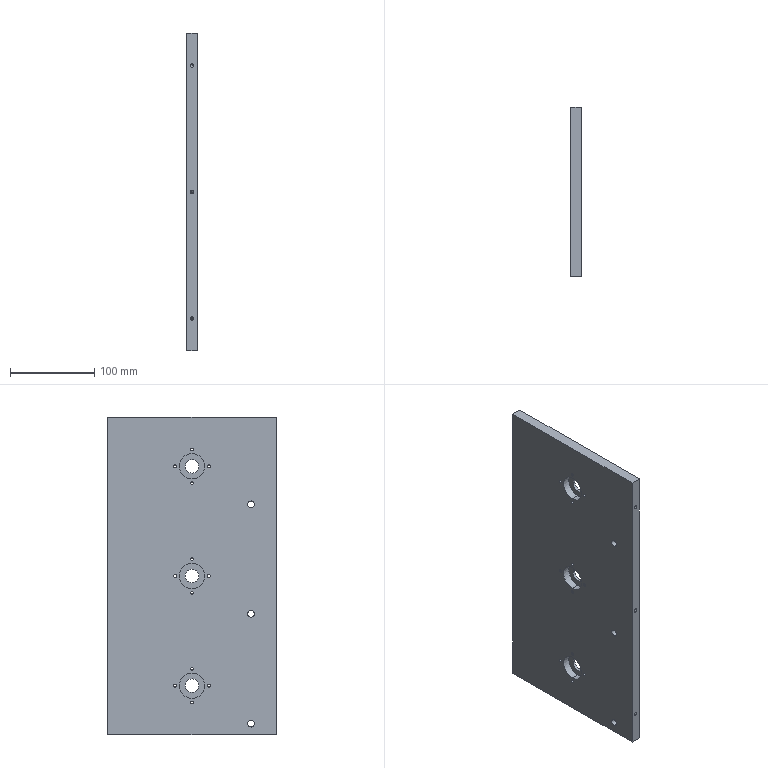Part | SolidWorks | features Cut 2, HoleWzd 2, Extrusion 1, ICE 1, MirrorPattern 1 | 1 solid | 75 faces | box 12 x 200 x 376 mm | volume 876393 mm3 | cylinder 54 | cone 12 | plane 9 | commonest cylinder face diameters 3.3 x24 4.2 x12 8 x6 16 x6 30 x6